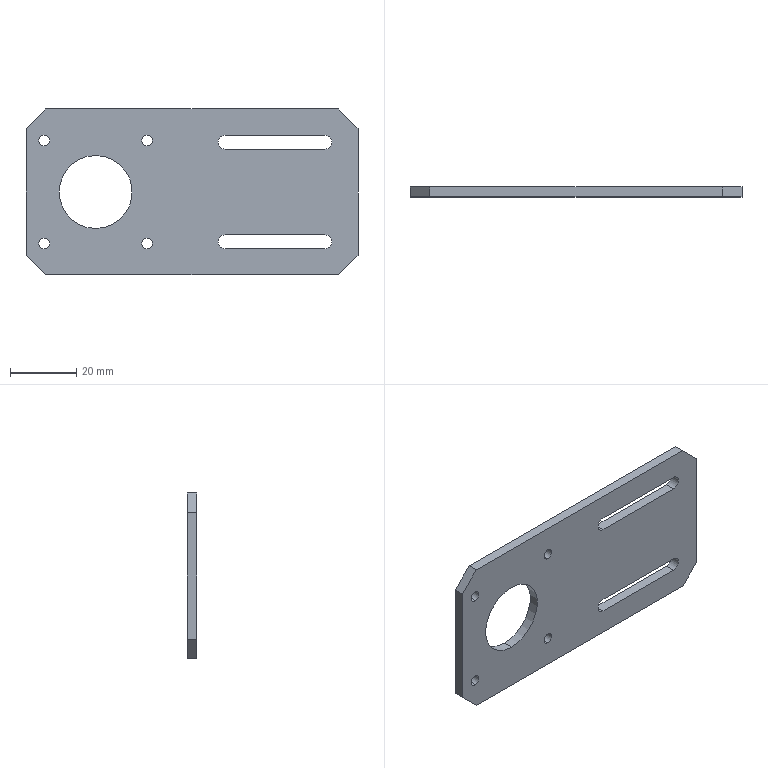Part | SolidWorks | features BaseBody 1 | 1 solid | 28 faces | box 100 x 3 x 50 mm | volume 12708 mm3 | cylinder 14 | plane 14 | commonest cylinder face diameters 3.2 x8 4.2 x4 22 x2
STEP:
#1=CARTESIAN_POINT('',(5.5,3.,-11.1));
#2=VERTEX_POINT('',#1);
#3=CARTESIAN_POINT('',(5.5,3.,-7.9));
#4=VERTEX_POINT('',#3);
#5=CARTESIAN_POINT('',(5.5,3.,-9.5));
#6=DIRECTION('',(0.,1.,0.));
#7=DIRECTION('',(0.,0.,-1.));
#8=AXIS2_PLACEMENT_3D('',#5,#6,#7);
#9=CIRCLE('',#8,1.6);
#10=EDGE_CURVE('',#2,#4,#9,.T.);
#11=ORIENTED_EDGE('',*,*,#10,.T.);
#12=CARTESIAN_POINT('',(5.5,0.,-7.9));
#13=VERTEX_POINT('',#12);
#14=CARTESIAN_POINT('',(5.5,3.,-7.9));
#15=DIRECTION('',(0.,-1.,0.));
#16=VECTOR('',#15,1000.);
#17=LINE('',#14,#16);
#18=EDGE_CURVE('',#4,#13,#17,.T.);
#19=ORIENTED_EDGE('',*,*,#18,.T.);
#20=CARTESIAN_POINT('',(5.5,0.,-11.1));
#21=VERTEX_POINT('',#20);
#22=CARTESIAN_POINT('',(5.5,0.,-9.5));
#23=DIRECTION('',(0.,1.,0.));
#24=DIRECTION('',(0.,0.,-1.));
#25=AXIS2_PLACEMENT_3D('',#22,#23,#24);
#26=CIRCLE('',#25,1.6);
#27=EDGE_CURVE('',#21,#13,#26,.T.);
#28=ORIENTED_EDGE('',*,*,#27,.F.);
#29=CARTESIAN_POINT('',(5.5,3.,-11.1));
#30=DIRECTION('',(0.,-1.,0.));
#31=VECTOR('',#30,1000.);
#32=LINE('',#29,#31);
#33=EDGE_CURVE('',#2,#21,#32,.T.);
#34=ORIENTED_EDGE('',*,*,#33,.F.);
#35=EDGE_LOOP('',(#11,#19,#28,#34));
#36=FACE_OUTER_BOUND('',#35,.T.);
#37=CARTESIAN_POINT('',(5.5,3.,-9.5));
#38=DIRECTION('',(0.,-1.,0.));
#39=DIRECTION('',(0.,0.,-1.));
#40=AXIS2_PLACEMENT_3D('',#37,#38,#39);
#41=CYLINDRICAL_SURFACE('',#40,1.6);
#42=ADVANCED_FACE('',(#36),#41,.F.);
#43=CARTESIAN_POINT('',(36.5,3.,-11.1));
#44=VERTEX_POINT('',#43);
#45=CARTESIAN_POINT('',(36.5,3.,-7.9));
#46=VERTEX_POINT('',#45);
#47=CARTESIAN_POINT('',(36.5,3.,-9.5));
#48=DIRECTION('',(0.,1.,0.));
#49=DIRECTION('',(0.,0.,-1.));
#50=AXIS2_PLACEMENT_3D('',#47,#48,#49);
#51=CIRCLE('',#50,1.6);
#52=EDGE_CURVE('',#44,#46,#51,.T.);
#53=ORIENTED_EDGE('',*,*,#52,.T.);
#54=CARTESIAN_POINT('',(36.5,0.,-7.9));
#55=VERTEX_POINT('',#54);
#56=CARTESIAN_POINT('',(36.5,3.,-7.9));
#57=DIRECTION('',(0.,-1.,0.));
#58=VECTOR('',#57,1000.);
#59=LINE('',#56,#58);
#60=EDGE_CURVE('',#46,#55,#59,.T.);
#61=ORIENTED_EDGE('',*,*,#60,.T.);
#62=CARTESIAN_POINT('',(36.5,0.,-11.1));
#63=VERTEX_POINT('',#62);
#64=CARTESIAN_POINT('',(36.5,0.,-9.5));
#65=DIRECTION('',(0.,1.,0.));
#66=DIRECTION('',(0.,0.,-1.));
#67=AXIS2_PLACEMENT_3D('',#64,#65,#66);
#68=CIRCLE('',#67,1.6);
#69=EDGE_CURVE('',#63,#55,#68,.T.);
#70=ORIENTED_EDGE('',*,*,#69,.F.);
#71=CARTESIAN_POINT('',(36.5,3.,-11.1));
#72=DIRECTION('',(0.,-1.,0.));
#73=VECTOR('',#72,1000.);
#74=LINE('',#71,#73);
#75=EDGE_CURVE('',#44,#63,#74,.T.);
#76=ORIENTED_EDGE('',*,*,#75,.F.);
#77=EDGE_LOOP('',(#53,#61,#70,#76));
#78=FACE_OUTER_BOUND('',#77,.T.);
#79=CARTESIAN_POINT('',(36.5,3.,-9.5));
#80=DIRECTION('',(0.,-1.,0.));
#81=DIRECTION('',(0.,0.,-1.));
#82=AXIS2_PLACEMENT_3D('',#79,#80,#81);
#83=CYLINDRICAL_SURFACE('',#82,1.6);
#84=ADVANCED_FACE('',(#78),#83,.F.);
#85=CARTESIAN_POINT('',(36.5,3.,-42.1));
#86=VERTEX_POINT('',#85);
#87=CARTESIAN_POINT('',(36.5,3.,-38.9));
#88=VERTEX_POINT('',#87);
#89=CARTESIAN_POINT('',(36.5,3.,-40.5));
#90=DIRECTION('',(0.,1.,0.));
#91=DIRECTION('',(0.,0.,-1.));
#92=AXIS2_PLACEMENT_3D('',#89,#90,#91);
#93=CIRCLE('',#92,1.6);
#94=EDGE_CURVE('',#86,#88,#93,.T.);
#95=ORIENTED_EDGE('',*,*,#94,.T.);
#96=CARTESIAN_POINT('',(36.5,0.,-38.9));
#97=VERTEX_POINT('',#96);
#98=CARTESIAN_POINT('',(36.5,3.,-38.9));
#99=DIRECTION('',(0.,-1.,0.));
#100=VECTOR('',#99,1000.);
#101=LINE('',#98,#100);
#102=EDGE_CURVE('',#88,#97,#101,.T.);
#103=ORIENTED_EDGE('',*,*,#102,.T.);
#104=CARTESIAN_POINT('',(36.5,0.,-42.1));
#105=VERTEX_POINT('',#104);
#106=CARTESIAN_POINT('',(36.5,0.,-40.5));
#107=DIRECTION('',(0.,1.,0.));
#108=DIRECTION('',(0.,0.,-1.));
#109=AXIS2_PLACEMENT_3D('',#106,#107,#108);
#110=CIRCLE('',#109,1.6);
#111=EDGE_CURVE('',#105,#97,#110,.T.);
#112=ORIENTED_EDGE('',*,*,#111,.F.);
#113=CARTESIAN_POINT('',(36.5,3.,-42.1));
#114=DIRECTION('',(0.,-1.,0.));
#115=VECTOR('',#114,1000.);
#116=LINE('',#113,#115);
#117=EDGE_CURVE('',#86,#105,#116,.T.);
#118=ORIENTED_EDGE('',*,*,#117,.F.);
#119=EDGE_LOOP('',(#95,#103,#112,#118));
#120=FACE_OUTER_BOUND('',#119,.T.);
#121=CARTESIAN_POINT('',(36.5,3.,-40.5));
#122=DIRECTION('',(0.,-1.,0.));
#123=DIRECTION('',(0.,0.,-1.));
#124=AXIS2_PLACEMENT_3D('',#121,#122,#123);
#125=CYLINDRICAL_SURFACE('',#124,1.6);
#126=ADVANCED_FACE('',(#120),#125,.F.);
#127=CARTESIAN_POINT('',(5.5,3.,-42.1));
#128=VERTEX_POINT('',#127);
#129=CARTESIAN_POINT('',(5.5,3.,-38.9));
#130=VERTEX_POINT('',#129);
#131=CARTESIAN_POINT('',(5.5,3.,-40.5));
#132=DIRECTION('',(0.,1.,0.));
#133=DIRECTION('',(0.,0.,-1.));
#134=AXIS2_PLACEMENT_3D('',#131,#132,#133);
#135=CIRCLE('',#134,1.6);
#136=EDGE_CURVE('',#128,#130,#135,.T.);
#137=ORIENTED_EDGE('',*,*,#136,.T.);
#138=CARTESIAN_POINT('',(5.5,0.,-38.9));
#139=VERTEX_POINT('',#138);
#140=CARTESIAN_POINT('',(5.5,3.,-38.9));
#141=DIRECTION('',(0.,-1.,0.));
#142=VECTOR('',#141,1000.);
#143=LINE('',#140,#142);
#144=EDGE_CURVE('',#130,#139,#143,.T.);
#145=ORIENTED_EDGE('',*,*,#144,.T.);
#146=CARTESIAN_POINT('',(5.5,0.,-42.1));
#147=VERTEX_POINT('',#146);
#148=CARTESIAN_POINT('',(5.5,0.,-40.5));
#149=DIRECTION('',(0.,1.,0.));
#150=DIRECTION('',(0.,0.,-1.));
#151=AXIS2_PLACEMENT_3D('',#148,#149,#150);
#152=CIRCLE('',#151,1.6);
#153=EDGE_CURVE('',#147,#139,#152,.T.);
#154=ORIENTED_EDGE('',*,*,#153,.F.);
#155=CARTESIAN_POINT('',(5.5,3.,-42.1));
#156=DIRECTION('',(0.,-1.,0.));
#157=VECTOR('',#156,1000.);
#158=LINE('',#155,#157);
#159=EDGE_CURVE('',#128,#147,#158,.T.);
#160=ORIENTED_EDGE('',*,*,#159,.F.);
#161=EDGE_LOOP('',(#137,#145,#154,#160));
#162=FACE_OUTER_BOUND('',#161,.T.);
#163=CARTESIAN_POINT('',(5.5,3.,-40.5));
#164=DIRECTION('',(0.,-1.,0.));
#165=DIRECTION('',(0.,0.,-1.));
#166=AXIS2_PLACEMENT_3D('',#163,#164,#165);
#167=CYLINDRICAL_SURFACE('',#166,1.6);
#168=ADVANCED_FACE('',(#162),#167,.F.);
#169=CARTESIAN_POINT('',(21.,3.,-36.));
#170=VERTEX_POINT('',#169);
#171=CARTESIAN_POINT('',(21.,3.,-14.));
#172=VERTEX_POINT('',#171);
#173=CARTESIAN_POINT('',(21.,3.,-25.));
#174=DIRECTION('',(0.,1.,0.));
#175=DIRECTION('',(0.,0.,-1.));
#176=AXIS2_PLACEMENT_3D('',#173,#174,#175);
#177=CIRCLE('',#176,11.);
#178=EDGE_CURVE('',#170,#172,#177,.T.);
#179=ORIENTED_EDGE('',*,*,#178,.T.);
#180=CARTESIAN_POINT('',(21.,0.,-14.));
#181=VERTEX_POINT('',#180);
#182=CARTESIAN_POINT('',(21.,3.,-14.));
#183=DIRECTION('',(0.,-1.,0.));
#184=VECTOR('',#183,1000.);
#185=LINE('',#182,#184);
#186=EDGE_CURVE('',#172,#181,#185,.T.);
#187=ORIENTED_EDGE('',*,*,#186,.T.);
#188=CARTESIAN_POINT('',(21.,0.,-36.));
#189=VERTEX_POINT('',#188);
#190=CARTESIAN_POINT('',(21.,0.,-25.));
#191=DIRECTION('',(0.,1.,0.));
#192=DIRECTION('',(0.,0.,-1.));
#193=AXIS2_PLACEMENT_3D('',#190,#191,#192);
#194=CIRCLE('',#193,11.);
#195=EDGE_CURVE('',#189,#181,#194,.T.);
#196=ORIENTED_EDGE('',*,*,#195,.F.);
#197=CARTESIAN_POINT('',(21.,3.,-36.));
#198=DIRECTION('',(0.,-1.,0.));
#199=VECTOR('',#198,1000.);
#200=LINE('',#197,#199);
#201=EDGE_CURVE('',#170,#189,#200,.T.);
#202=ORIENTED_EDGE('',*,*,#201,.F.);
#203=EDGE_LOOP('',(#179,#187,#196,#202));
#204=FACE_OUTER_BOUND('',#203,.T.);
#205=CARTESIAN_POINT('',(21.,3.,-25.));
#206=DIRECTION('',(0.,-1.,0.));
#207=DIRECTION('',(0.,0.,-1.));
#208=AXIS2_PLACEMENT_3D('',#205,#206,#207);
#209=CYLINDRICAL_SURFACE('',#208,11.);
#210=ADVANCED_FACE('',(#204),#209,.F.);
#211=CARTESIAN_POINT('',(90.,3.,-12.1));
#212=VERTEX_POINT('',#211);
#213=CARTESIAN_POINT('',(60.,3.,-12.1));
#214=VERTEX_POINT('',#213);
#215=CARTESIAN_POINT('',(0.,3.,-12.1));
#216=DIRECTION('',(-1.,0.,0.));
#217=VECTOR('',#216,1000.);
#218=LINE('',#215,#217);
#219=EDGE_CURVE('',#212,#214,#218,.T.);
#220=ORIENTED_EDGE('',*,*,#219,.F.);
#221=CARTESIAN_POINT('',(90.,3.,-7.9));
#222=VERTEX_POINT('',#221);
#223=CARTESIAN_POINT('',(90.,3.,-10.));
#224=DIRECTION('',(0.,1.,0.));
#225=DIRECTION('',(0.,0.,-1.));
#226=AXIS2_PLACEMENT_3D('',#223,#224,#225);
#227=CIRCLE('',#226,2.1);
#228=EDGE_CURVE('',#222,#212,#227,.T.);
#229=ORIENTED_EDGE('',*,*,#228,.F.);
#230=CARTESIAN_POINT('',(60.,3.,-7.9));
#231=VERTEX_POINT('',#230);
#232=CARTESIAN_POINT('',(0.,3.,-7.9));
#233=DIRECTION('',(1.,0.,0.));
#234=VECTOR('',#233,1000.);
#235=LINE('',#232,#234);
#236=EDGE_CURVE('',#231,#222,#235,.T.);
#237=ORIENTED_EDGE('',*,*,#236,.F.);
#238=CARTESIAN_POINT('',(60.,3.,-10.));
#239=DIRECTION('',(0.,1.,0.));
#240=DIRECTION('',(0.,0.,-1.));
#241=AXIS2_PLACEMENT_3D('',#238,#239,#240);
#242=CIRCLE('',#241,2.1);
#243=EDGE_CURVE('',#214,#231,#242,.T.);
#244=ORIENTED_EDGE('',*,*,#243,.F.);
#245=EDGE_LOOP('',(#220,#229,#237,#244));
#246=FACE_BOUND('',#245,.T.);
#247=ORIENTED_EDGE('',*,*,#10,.F.);
#248=CARTESIAN_POINT('',(5.5,3.,-9.5));
#249=DIRECTION('',(0.,1.,0.));
#250=DIRECTION('',(0.,0.,-1.));
#251=AXIS2_PLACEMENT_3D('',#248,#249,#250);
#252=CIRCLE('',#251,1.6);
#253=EDGE_CURVE('',#4,#2,#252,.T.);
#254=ORIENTED_EDGE('',*,*,#253,.F.);
#255=EDGE_LOOP('',(#247,#254));
#256=FACE_BOUND('',#255,.T.);
#257=ORIENTED_EDGE('',*,*,#52,.F.);
#258=CARTESIAN_POINT('',(36.5,3.,-9.5));
#259=DIRECTION('',(0.,1.,0.));
#260=DIRECTION('',(0.,0.,-1.));
#261=AXIS2_PLACEMENT_3D('',#258,#259,#260);
#262=CIRCLE('',#261,1.6);
#263=EDGE_CURVE('',#46,#44,#262,.T.);
#264=ORIENTED_EDGE('',*,*,#263,.F.);
#265=EDGE_LOOP('',(#257,#264));
#266=FACE_BOUND('',#265,.T.);
#267=ORIENTED_EDGE('',*,*,#94,.F.);
#268=CARTESIAN_POINT('',(36.5,3.,-40.5));
#269=DIRECTION('',(0.,1.,0.));
#270=DIRECTION('',(0.,0.,-1.));
#271=AXIS2_PLACEMENT_3D('',#268,#269,#270);
#272=CIRCLE('',#271,1.6);
#273=EDGE_CURVE('',#88,#86,#272,.T.);
#274=ORIENTED_EDGE('',*,*,#273,.F.);
#275=EDGE_LOOP('',(#267,#274));
#276=FACE_BOUND('',#275,.T.);
#277=ORIENTED_EDGE('',*,*,#136,.F.);
#278=CARTESIAN_POINT('',(5.5,3.,-40.5));
#279=DIRECTION('',(0.,1.,0.));
#280=DIRECTION('',(0.,0.,-1.));
#281=AXIS2_PLACEMENT_3D('',#278,#279,#280);
#282=CIRCLE('',#281,1.6);
#283=EDGE_CURVE('',#130,#128,#282,.T.);
#284=ORIENTED_EDGE('',*,*,#283,.F.);
#285=EDGE_LOOP('',(#277,#284));
#286=FACE_BOUND('',#285,.T.);
#287=ORIENTED_EDGE('',*,*,#178,.F.);
#288=CARTESIAN_POINT('',(21.,3.,-25.));
#289=DIRECTION('',(0.,1.,0.));
#290=DIRECTION('',(0.,0.,-1.));
#291=AXIS2_PLACEMENT_3D('',#288,#289,#290);
#292=CIRCLE('',#291,11.);
#293=EDGE_CURVE('',#172,#170,#292,.T.);
#294=ORIENTED_EDGE('',*,*,#293,.F.);
#295=EDGE_LOOP('',(#287,#294));
#296=FACE_BOUND('',#295,.T.);
#297=CARTESIAN_POINT('',(6.,3.,0.));
#298=VERTEX_POINT('',#297);
#299=CARTESIAN_POINT('',(0.,3.,-6.));
#300=VERTEX_POINT('',#299);
#301=CARTESIAN_POINT('',(6.,3.,0.));
#302=DIRECTION('',(-0.7071,0.,-0.7071));
#303=VECTOR('',#302,1000.);
#304=LINE('',#301,#303);
#305=EDGE_CURVE('',#298,#300,#304,.T.);
#306=ORIENTED_EDGE('',*,*,#305,.F.);
#307=CARTESIAN_POINT('',(94.,3.,0.));
#308=VERTEX_POINT('',#307);
#309=CARTESIAN_POINT('',(0.,3.,0.));
#310=DIRECTION('',(-1.,0.,0.));
#311=VECTOR('',#310,1000.);
#312=LINE('',#309,#311);
#313=EDGE_CURVE('',#308,#298,#312,.T.);
#314=ORIENTED_EDGE('',*,*,#313,.F.);
#315=CARTESIAN_POINT('',(100.,3.,-6.));
#316=VERTEX_POINT('',#315);
#317=CARTESIAN_POINT('',(100.,3.,-6.));
#318=DIRECTION('',(-0.7071,0.,0.7071));
#319=VECTOR('',#318,1000.);
#320=LINE('',#317,#319);
#321=EDGE_CURVE('',#316,#308,#320,.T.);
#322=ORIENTED_EDGE('',*,*,#321,.F.);
#323=CARTESIAN_POINT('',(100.,3.,-44.));
#324=VERTEX_POINT('',#323);
#325=CARTESIAN_POINT('',(100.,3.,0.));
#326=DIRECTION('',(0.,0.,1.));
#327=VECTOR('',#326,1000.);
#328=LINE('',#325,#327);
#329=EDGE_CURVE('',#324,#316,#328,.T.);
#330=ORIENTED_EDGE('',*,*,#329,.F.);
#331=CARTESIAN_POINT('',(94.,3.,-50.));
#332=VERTEX_POINT('',#331);
#333=CARTESIAN_POINT('',(94.,3.,-50.));
#334=DIRECTION('',(0.7071,0.,0.7071));
#335=VECTOR('',#334,1000.);
#336=LINE('',#333,#335);
#337=EDGE_CURVE('',#332,#324,#336,.T.);
#338=ORIENTED_EDGE('',*,*,#337,.F.);
#339=CARTESIAN_POINT('',(6.,3.,-50.));
#340=VERTEX_POINT('',#339);
#341=CARTESIAN_POINT('',(0.,3.,-50.));
#342=DIRECTION('',(1.,0.,0.));
#343=VECTOR('',#342,1000.);
#344=LINE('',#341,#343);
#345=EDGE_CURVE('',#340,#332,#344,.T.);
#346=ORIENTED_EDGE('',*,*,#345,.F.);
#347=CARTESIAN_POINT('',(0.,3.,-44.));
#348=VERTEX_POINT('',#347);
#349=CARTESIAN_POINT('',(0.,3.,-44.));
#350=DIRECTION('',(0.7071,0.,-0.7071));
#351=VECTOR('',#350,1000.);
#352=LINE('',#349,#351);
#353=EDGE_CURVE('',#348,#340,#352,.T.);
#354=ORIENTED_EDGE('',*,*,#353,.F.);
#355=CARTESIAN_POINT('',(0.,3.,0.));
#356=DIRECTION('',(0.,0.,-1.));
#357=VECTOR('',#356,1000.);
#358=LINE('',#355,#357);
#359=EDGE_CURVE('',#300,#348,#358,.T.);
#360=ORIENTED_EDGE('',*,*,#359,.F.);
#361=EDGE_LOOP('',(#306,#314,#322,#330,#338,#346,#354,#360));
#362=FACE_OUTER_BOUND('',#361,.T.);
#363=CARTESIAN_POINT('',(90.,3.,-42.1));
#364=VERTEX_POINT('',#363);
#365=CARTESIAN_POINT('',(60.,3.,-42.1));
#366=VERTEX_POINT('',#365);
#367=CARTESIAN_POINT('',(0.,3.,-42.1));
#368=DIRECTION('',(-1.,0.,0.));
#369=VECTOR('',#368,1000.);
#370=LINE('',#367,#369);
#371=EDGE_CURVE('',#364,#366,#370,.T.);
#372=ORIENTED_EDGE('',*,*,#371,.F.);
#373=CARTESIAN_POINT('',(90.,3.,-37.9));
#374=VERTEX_POINT('',#373);
#375=CARTESIAN_POINT('',(90.,3.,-40.));
#376=DIRECTION('',(0.,1.,0.));
#377=DIRECTION('',(0.,0.,-1.));
#378=AXIS2_PLACEMENT_3D('',#375,#376,#377);
#379=CIRCLE('',#378,2.1);
#380=EDGE_CURVE('',#374,#364,#379,.T.);
#381=ORIENTED_EDGE('',*,*,#380,.F.);
#382=CARTESIAN_POINT('',(60.,3.,-37.9));
#383=VERTEX_POINT('',#382);
#384=CARTESIAN_POINT('',(0.,3.,-37.9));
#385=DIRECTION('',(1.,0.,0.));
#386=VECTOR('',#385,1000.);
#387=LINE('',#384,#386);
#388=EDGE_CURVE('',#383,#374,#387,.T.);
#389=ORIENTED_EDGE('',*,*,#388,.F.);
#390=CARTESIAN_POINT('',(60.,3.,-40.));
#391=DIRECTION('',(0.,1.,0.));
#392=DIRECTION('',(0.,0.,-1.));
#393=AXIS2_PLACEMENT_3D('',#390,#391,#392);
#394=CIRCLE('',#393,2.1);
#395=EDGE_CURVE('',#366,#383,#394,.T.);
#396=ORIENTED_EDGE('',*,*,#395,.F.);
#397=EDGE_LOOP('',(#372,#381,#389,#396));
#398=FACE_BOUND('',#397,.T.);
#399=CARTESIAN_POINT('',(0.,3.,0.));
#400=DIRECTION('',(0.,-1.,0.));
#401=DIRECTION('',(0.,0.,-1.));
#402=AXIS2_PLACEMENT_3D('',#399,#400,#401);
#403=PLANE('',#402);
#404=ADVANCED_FACE('',(#246,#256,#266,#276,#286,#296,#362,#398),#403,.F.);
#405=CARTESIAN_POINT('',(60.,0.,-12.1));
#406=VERTEX_POINT('',#405);
#407=CARTESIAN_POINT('',(60.,3.,-12.1));
#408=DIRECTION('',(0.,-1.,0.));
#409=VECTOR('',#408,1000.);
#410=LINE('',#407,#409);
#411=EDGE_CURVE('',#214,#406,#410,.T.);
#412=ORIENTED_EDGE('',*,*,#411,.F.);
#413=ORIENTED_EDGE('',*,*,#243,.T.);
#414=CARTESIAN_POINT('',(60.,0.,-7.9));
#415=VERTEX_POINT('',#414);
#416=CARTESIAN_POINT('',(60.,3.,-7.9));
#417=DIRECTION('',(0.,1.,0.));
#418=VECTOR('',#417,1000.);
#419=LINE('',#416,#418);
#420=EDGE_CURVE('',#415,#231,#419,.T.);
#421=ORIENTED_EDGE('',*,*,#420,.F.);
#422=CARTESIAN_POINT('',(60.,0.,-10.));
#423=DIRECTION('',(0.,1.,0.));
#424=DIRECTION('',(0.,0.,-1.));
#425=AXIS2_PLACEMENT_3D('',#422,#423,#424);
#426=CIRCLE('',#425,2.1);
#427=EDGE_CURVE('',#406,#415,#426,.T.);
#428=ORIENTED_EDGE('',*,*,#427,.F.);
#429=EDGE_LOOP('',(#412,#413,#421,#428));
#430=FACE_OUTER_BOUND('',#429,.T.);
#431=CARTESIAN_POINT('',(60.,3.,-10.));
#432=DIRECTION('',(0.,-1.,0.));
#433=DIRECTION('',(0.,0.,-1.));
#434=AXIS2_PLACEMENT_3D('',#431,#432,#433);
#435=CYLINDRICAL_SURFACE('',#434,2.1);
#436=ADVANCED_FACE('',(#430),#435,.F.);
#437=ORIENTED_EDGE('',*,*,#219,.T.);
#438=ORIENTED_EDGE('',*,*,#411,.T.);
#439=CARTESIAN_POINT('',(90.,0.,-12.1));
#440=VERTEX_POINT('',#439);
#441=CARTESIAN_POINT('',(60.,0.,-12.1));
#442=DIRECTION('',(1.,0.,0.));
#443=VECTOR('',#442,1000.);
#444=LINE('',#441,#443);
#445=EDGE_CURVE('',#406,#440,#444,.T.);
#446=ORIENTED_EDGE('',*,*,#445,.T.);
#447=CARTESIAN_POINT('',(90.,3.,-12.1));
#448=DIRECTION('',(0.,1.,0.));
#449=VECTOR('',#448,1000.);
#450=LINE('',#447,#449);
#451=EDGE_CURVE('',#440,#212,#450,.T.);
#452=ORIENTED_EDGE('',*,*,#451,.T.);
#453=EDGE_LOOP('',(#437,#438,#446,#452));
#454=FACE_OUTER_BOUND('',#453,.T.);
#455=CARTESIAN_POINT('',(60.,3.,-12.1));
#456=DIRECTION('',(0.,0.,1.));
#457=DIRECTION('',(1.,0.,0.));
#458=AXIS2_PLACEMENT_3D('',#455,#456,#457);
#459=PLANE('',#458);
#460=ADVANCED_FACE('',(#454),#459,.T.);
#461=CARTESIAN_POINT('',(90.,0.,-7.9));
#462=VERTEX_POINT('',#461);
#463=CARTESIAN_POINT('',(90.,3.,-7.9));
#464=DIRECTION('',(0.,-1.,0.));
#465=VECTOR('',#464,1000.);
#466=LINE('',#463,#465);
#467=EDGE_CURVE('',#222,#462,#466,.T.);
#468=ORIENTED_EDGE('',*,*,#467,.F.);
#469=ORIENTED_EDGE('',*,*,#228,.T.);
#470=ORIENTED_EDGE('',*,*,#451,.F.);
#471=CARTESIAN_POINT('',(90.,0.,-10.));
#472=DIRECTION('',(0.,1.,0.));
#473=DIRECTION('',(0.,0.,-1.));
#474=AXIS2_PLACEMENT_3D('',#471,#472,#473);
#475=CIRCLE('',#474,2.1);
#476=EDGE_CURVE('',#462,#440,#475,.T.);
#477=ORIENTED_EDGE('',*,*,#476,.F.);
#478=EDGE_LOOP('',(#468,#469,#470,#477));
#479=FACE_OUTER_BOUND('',#478,.T.);
#480=CARTESIAN_POINT('',(90.,3.,-10.));
#481=DIRECTION('',(0.,-1.,0.));
#482=DIRECTION('',(0.,0.,-1.));
#483=AXIS2_PLACEMENT_3D('',#480,#481,#482);
#484=CYLINDRICAL_SURFACE('',#483,2.1);
#485=ADVANCED_FACE('',(#479),#484,.F.);
#486=ORIENTED_EDGE('',*,*,#236,.T.);
#487=ORIENTED_EDGE('',*,*,#467,.T.);
#488=CARTESIAN_POINT('',(60.,0.,-7.9));
#489=DIRECTION('',(-1.,0.,0.));
#490=VECTOR('',#489,1000.);
#491=LINE('',#488,#490);
#492=EDGE_CURVE('',#462,#415,#491,.T.);
#493=ORIENTED_EDGE('',*,*,#492,.T.);
#494=ORIENTED_EDGE('',*,*,#420,.T.);
#495=EDGE_LOOP('',(#486,#487,#493,#494));
#496=FACE_OUTER_BOUND('',#495,.T.);
#497=CARTESIAN_POINT('',(60.,3.,-7.9));
#498=DIRECTION('',(0.,0.,-1.));
#499=DIRECTION('',(-1.,0.,0.));
#500=AXIS2_PLACEMENT_3D('',#497,#498,#499);
#501=PLANE('',#500);
#502=ADVANCED_FACE('',(#496),#501,.T.);
#503=ORIENTED_EDGE('',*,*,#18,.F.);
#504=ORIENTED_EDGE('',*,*,#253,.T.);
#505=ORIENTED_EDGE('',*,*,#33,.T.);
#506=CARTESIAN_POINT('',(5.5,0.,-9.5));
#507=DIRECTION('',(0.,1.,0.));
#508=DIRECTION('',(0.,0.,-1.));
#509=AXIS2_PLACEMENT_3D('',#506,#507,#508);
#510=CIRCLE('',#509,1.6);
#511=EDGE_CURVE('',#13,#21,#510,.T.);
#512=ORIENTED_EDGE('',*,*,#511,.F.);
#513=EDGE_LOOP('',(#503,#504,#505,#512));
#514=FACE_OUTER_BOUND('',#513,.T.);
#515=CARTESIAN_POINT('',(5.5,3.,-9.5));
#516=DIRECTION('',(0.,-1.,0.));
#517=DIRECTION('',(0.,0.,-1.));
#518=AXIS2_PLACEMENT_3D('',#515,#516,#517);
#519=CYLINDRICAL_SURFACE('',#518,1.6);
#520=ADVANCED_FACE('',(#514),#519,.F.);
#521=ORIENTED_EDGE('',*,*,#60,.F.);
#522=ORIENTED_EDGE('',*,*,#263,.T.);
#523=ORIENTED_EDGE('',*,*,#75,.T.);
#524=CARTESIAN_POINT('',(36.5,0.,-9.5));
#525=DIRECTION('',(0.,1.,0.));
#526=DIRECTION('',(0.,0.,-1.));
#527=AXIS2_PLACEMENT_3D('',#524,#525,#526);
#528=CIRCLE('',#527,1.6);
#529=EDGE_CURVE('',#55,#63,#528,.T.);
#530=ORIENTED_EDGE('',*,*,#529,.F.);
#531=EDGE_LOOP('',(#521,#522,#523,#530));
#532=FACE_OUTER_BOUND('',#531,.T.);
#533=CARTESIAN_POINT('',(36.5,3.,-9.5));
#534=DIRECTION('',(0.,-1.,0.));
#535=DIRECTION('',(0.,0.,-1.));
#536=AXIS2_PLACEMENT_3D('',#533,#534,#535);
#537=CYLINDRICAL_SURFACE('',#536,1.6);
#538=ADVANCED_FACE('',(#532),#537,.F.);
#539=ORIENTED_EDGE('',*,*,#102,.F.);
#540=ORIENTED_EDGE('',*,*,#273,.T.);
#541=ORIENTED_EDGE('',*,*,#117,.T.);
#542=CARTESIAN_POINT('',(36.5,0.,-40.5));
#543=DIRECTION('',(0.,1.,0.));
#544=DIRECTION('',(0.,0.,-1.));
#545=AXIS2_PLACEMENT_3D('',#542,#543,#544);
#546=CIRCLE('',#545,1.6);
#547=EDGE_CURVE('',#97,#105,#546,.T.);
#548=ORIENTED_EDGE('',*,*,#547,.F.);
#549=EDGE_LOOP('',(#539,#540,#541,#548));
#550=FACE_OUTER_BOUND('',#549,.T.);
#551=CARTESIAN_POINT('',(36.5,3.,-40.5));
#552=DIRECTION('',(0.,-1.,0.));
#553=DIRECTION('',(0.,0.,-1.));
#554=AXIS2_PLACEMENT_3D('',#551,#552,#553);
#555=CYLINDRICAL_SURFACE('',#554,1.6);
#556=ADVANCED_FACE('',(#550),#555,.F.);
#557=ORIENTED_EDGE('',*,*,#144,.F.);
#558=ORIENTED_EDGE('',*,*,#283,.T.);
#559=ORIENTED_EDGE('',*,*,#159,.T.);
#560=CARTESIAN_POINT('',(5.5,0.,-40.5));
#561=DIRECTION('',(0.,1.,0.));
#562=DIRECTION('',(0.,0.,-1.));
#563=AXIS2_PLACEMENT_3D('',#560,#561,#562);
#564=CIRCLE('',#563,1.6);
#565=EDGE_CURVE('',#139,#147,#564,.T.);
#566=ORIENTED_EDGE('',*,*,#565,.F.);
#567=EDGE_LOOP('',(#557,#558,#559,#566));
#568=FACE_OUTER_BOUND('',#567,.T.);
#569=CARTESIAN_POINT('',(5.5,3.,-40.5));
#570=DIRECTION('',(0.,-1.,0.));
#571=DIRECTION('',(0.,0.,-1.));
#572=AXIS2_PLACEMENT_3D('',#569,#570,#571);
#573=CYLINDRICAL_SURFACE('',#572,1.6);
#574=ADVANCED_FACE('',(#568),#573,.F.);
#575=ORIENTED_EDGE('',*,*,#186,.F.);
#576=ORIENTED_EDGE('',*,*,#293,.T.);
#577=ORIENTED_EDGE('',*,*,#201,.T.);
#578=CARTESIAN_POINT('',(21.,0.,-25.));
#579=DIRECTION('',(0.,1.,0.));
#580=DIRECTION('',(0.,0.,-1.));
#581=AXIS2_PLACEMENT_3D('',#578,#579,#580);
#582=CIRCLE('',#581,11.);
#583=EDGE_CURVE('',#181,#189,#582,.T.);
#584=ORIENTED_EDGE('',*,*,#583,.F.);
#585=EDGE_LOOP('',(#575,#576,#577,#584));
#586=FACE_OUTER_BOUND('',#585,.T.);
#587=CARTESIAN_POINT('',(21.,3.,-25.));
#588=DIRECTION('',(0.,-1.,0.));
#589=DIRECTION('',(0.,0.,-1.));
#590=AXIS2_PLACEMENT_3D('',#587,#588,#589);
#591=CYLINDRICAL_SURFACE('',#590,11.);
#592=ADVANCED_FACE('',(#586),#591,.F.);
#593=CARTESIAN_POINT('',(0.,0.,-6.));
#594=VERTEX_POINT('',#593);
#595=CARTESIAN_POINT('',(0.,3.,-6.));
#596=DIRECTION('',(0.,-1.,0.));
#597=VECTOR('',#596,1000.);
#598=LINE('',#595,#597);
#599=EDGE_CURVE('',#300,#594,#598,.T.);
#600=ORIENTED_EDGE('',*,*,#599,.F.);
#601=ORIENTED_EDGE('',*,*,#359,.T.);
#602=CARTESIAN_POINT('',(0.,0.,-44.));
#603=VERTEX_POINT('',#602);
#604=CARTESIAN_POINT('',(0.,3.,-44.));
#605=DIRECTION('',(0.,1.,0.));
#606=VECTOR('',#605,1000.);
#607=LINE('',#604,#606);
#608=EDGE_CURVE('',#603,#348,#607,.T.);
#609=ORIENTED_EDGE('',*,*,#608,.F.);
#610=CARTESIAN_POINT('',(0.,0.,0.));
#611=DIRECTION('',(0.,0.,-1.));
#612=VECTOR('',#611,1000.);
#613=LINE('',#610,#612);
#614=EDGE_CURVE('',#594,#603,#613,.T.);
#615=ORIENTED_EDGE('',*,*,#614,.F.);
#616=EDGE_LOOP('',(#600,#601,#609,#615));
#617=FACE_OUTER_BOUND('',#616,.T.);
#618=CARTESIAN_POINT('',(0.,3.,0.));
#619=DIRECTION('',(1.,0.,0.));
#620=DIRECTION('',(0.,0.,-1.));
#621=AXIS2_PLACEMENT_3D('',#618,#619,#620);
#622=PLANE('',#621);
#623=ADVANCED_FACE('',(#617),#622,.F.);
#624=ORIENTED_EDGE('',*,*,#599,.T.);
#625=CARTESIAN_POINT('',(6.,0.,0.));
#626=VERTEX_POINT('',#625);
#627=CARTESIAN_POINT('',(6.,0.,0.));
#628=DIRECTION('',(-0.7071,0.,-0.7071));
#629=VECTOR('',#628,1000.);
#630=LINE('',#627,#629);
#631=EDGE_CURVE('',#626,#594,#630,.T.);
#632=ORIENTED_EDGE('',*,*,#631,.F.);
#633=CARTESIAN_POINT('',(6.,3.,0.));
#634=DIRECTION('',(0.,-1.,0.));
#635=VECTOR('',#634,1000.);
#636=LINE('',#633,#635);
#637=EDGE_CURVE('',#298,#626,#636,.T.);
#638=ORIENTED_EDGE('',*,*,#637,.F.);
#639=ORIENTED_EDGE('',*,*,#305,.T.);
#640=EDGE_LOOP('',(#624,#632,#638,#639));
#641=FACE_OUTER_BOUND('',#640,.T.);
#642=CARTESIAN_POINT('',(6.,3.,0.));
#643=DIRECTION('',(0.7071,0.,-0.7071));
#644=DIRECTION('',(-0.7071,0.,-0.7071));
#645=AXIS2_PLACEMENT_3D('',#642,#643,#644);
#646=PLANE('',#645);
#647=ADVANCED_FACE('',(#641),#646,.F.);
#648=ORIENTED_EDGE('',*,*,#637,.T.);
#649=CARTESIAN_POINT('',(94.,0.,0.));
#650=VERTEX_POINT('',#649);
#651=CARTESIAN_POINT('',(0.,0.,0.));
#652=DIRECTION('',(-1.,0.,0.));
#653=VECTOR('',#652,1000.);
#654=LINE('',#651,#653);
#655=EDGE_CURVE('',#650,#626,#654,.T.);
#656=ORIENTED_EDGE('',*,*,#655,.F.);
#657=CARTESIAN_POINT('',(94.,3.,0.));
#658=DIRECTION('',(0.,-1.,0.));
#659=VECTOR('',#658,1000.);
#660=LINE('',#657,#659);
#661=EDGE_CURVE('',#308,#650,#660,.T.);
#662=ORIENTED_EDGE('',*,*,#661,.F.);
#663=ORIENTED_EDGE('',*,*,#313,.T.);
#664=EDGE_LOOP('',(#648,#656,#662,#663));
#665=FACE_OUTER_BOUND('',#664,.T.);
#666=CARTESIAN_POINT('',(0.,3.,0.));
#667=DIRECTION('',(0.,0.,-1.));
#668=DIRECTION('',(-1.,0.,0.));
#669=AXIS2_PLACEMENT_3D('',#666,#667,#668);
#670=PLANE('',#669);
#671=ADVANCED_FACE('',(#665),#670,.F.);
#672=ORIENTED_EDGE('',*,*,#661,.T.);
#673=CARTESIAN_POINT('',(100.,0.,-6.));
#674=VERTEX_POINT('',#673);
#675=CARTESIAN_POINT('',(100.,0.,-6.));
#676=DIRECTION('',(-0.7071,0.,0.7071));
#677=VECTOR('',#676,1000.);
#678=LINE('',#675,#677);
#679=EDGE_CURVE('',#674,#650,#678,.T.);
#680=ORIENTED_EDGE('',*,*,#679,.F.);
#681=CARTESIAN_POINT('',(100.,3.,-6.));
#682=DIRECTION('',(0.,-1.,0.));
#683=VECTOR('',#682,1000.);
#684=LINE('',#681,#683);
#685=EDGE_CURVE('',#316,#674,#684,.T.);
#686=ORIENTED_EDGE('',*,*,#685,.F.);
#687=ORIENTED_EDGE('',*,*,#321,.T.);
#688=EDGE_LOOP('',(#672,#680,#686,#687));
#689=FACE_OUTER_BOUND('',#688,.T.);
#690=CARTESIAN_POINT('',(100.,3.,-6.));
#691=DIRECTION('',(-0.7071,0.,-0.7071));
#692=DIRECTION('',(-0.7071,0.,0.7071));
#693=AXIS2_PLACEMENT_3D('',#690,#691,#692);
#694=PLANE('',#693);
#695=ADVANCED_FACE('',(#689),#694,.F.);
#696=CARTESIAN_POINT('',(100.,0.,-44.));
#697=VERTEX_POINT('',#696);
#698=CARTESIAN_POINT('',(100.,3.,-44.));
#699=DIRECTION('',(0.,-1.,0.));
#700=VECTOR('',#699,1000.);
#701=LINE('',#698,#700);
#702=EDGE_CURVE('',#324,#697,#701,.T.);
#703=ORIENTED_EDGE('',*,*,#702,.F.);
#704=ORIENTED_EDGE('',*,*,#329,.T.);
#705=ORIENTED_EDGE('',*,*,#685,.T.);
#706=CARTESIAN_POINT('',(100.,0.,0.));
#707=DIRECTION('',(0.,0.,1.));
#708=VECTOR('',#707,1000.);
#709=LINE('',#706,#708);
#710=EDGE_CURVE('',#697,#674,#709,.T.);
#711=ORIENTED_EDGE('',*,*,#710,.F.);
#712=EDGE_LOOP('',(#703,#704,#705,#711));
#713=FACE_OUTER_BOUND('',#712,.T.);
#714=CARTESIAN_POINT('',(100.,3.,0.));
#715=DIRECTION('',(-1.,0.,0.));
#716=DIRECTION('',(0.,0.,1.));
#717=AXIS2_PLACEMENT_3D('',#714,#715,#716);
#718=PLANE('',#717);
#719=ADVANCED_FACE('',(#713),#718,.F.);
#720=ORIENTED_EDGE('',*,*,#702,.T.);
#721=CARTESIAN_POINT('',(94.,0.,-50.));
#722=VERTEX_POINT('',#721);
#723=CARTESIAN_POINT('',(94.,0.,-50.));
#724=DIRECTION('',(0.7071,0.,0.7071));
#725=VECTOR('',#724,1000.);
#726=LINE('',#723,#725);
#727=EDGE_CURVE('',#722,#697,#726,.T.);
#728=ORIENTED_EDGE('',*,*,#727,.F.);
#729=CARTESIAN_POINT('',(94.,3.,-50.));
#730=DIRECTION('',(0.,-1.,0.));
#731=VECTOR('',#730,1000.);
#732=LINE('',#729,#731);
#733=EDGE_CURVE('',#332,#722,#732,.T.);
#734=ORIENTED_EDGE('',*,*,#733,.F.);
#735=ORIENTED_EDGE('',*,*,#337,.T.);
#736=EDGE_LOOP('',(#720,#728,#734,#735));
#737=FACE_OUTER_BOUND('',#736,.T.);
#738=CARTESIAN_POINT('',(94.,3.,-50.));
#739=DIRECTION('',(-0.7071,0.,0.7071));
#740=DIRECTION('',(0.7071,0.,0.7071));
#741=AXIS2_PLACEMENT_3D('',#738,#739,#740);
#742=PLANE('',#741);
#743=ADVANCED_FACE('',(#737),#742,.F.);
#744=CARTESIAN_POINT('',(6.,0.,-50.));
#745=VERTEX_POINT('',#744);
#746=CARTESIAN_POINT('',(6.,3.,-50.));
#747=DIRECTION('',(0.,-1.,0.));
#748=VECTOR('',#747,1000.);
#749=LINE('',#746,#748);
#750=EDGE_CURVE('',#340,#745,#749,.T.);
#751=ORIENTED_EDGE('',*,*,#750,.F.);
#752=ORIENTED_EDGE('',*,*,#345,.T.);
#753=ORIENTED_EDGE('',*,*,#733,.T.);
#754=CARTESIAN_POINT('',(0.,0.,-50.));
#755=DIRECTION('',(1.,0.,0.));
#756=VECTOR('',#755,1000.);
#757=LINE('',#754,#756);
#758=EDGE_CURVE('',#745,#722,#757,.T.);
#759=ORIENTED_EDGE('',*,*,#758,.F.);
#760=EDGE_LOOP('',(#751,#752,#753,#759));
#761=FACE_OUTER_BOUND('',#760,.T.);
#762=CARTESIAN_POINT('',(0.,3.,-50.));
#763=DIRECTION('',(0.,0.,1.));
#764=DIRECTION('',(1.,0.,0.));
#765=AXIS2_PLACEMENT_3D('',#762,#763,#764);
#766=PLANE('',#765);
#767=ADVANCED_FACE('',(#761),#766,.F.);
#768=ORIENTED_EDGE('',*,*,#750,.T.);
#769=CARTESIAN_POINT('',(0.,0.,-44.));
#770=DIRECTION('',(0.7071,0.,-0.7071));
#771=VECTOR('',#770,1000.);
#772=LINE('',#769,#771);
#773=EDGE_CURVE('',#603,#745,#772,.T.);
#774=ORIENTED_EDGE('',*,*,#773,.F.);
#775=ORIENTED_EDGE('',*,*,#608,.T.);
#776=ORIENTED_EDGE('',*,*,#353,.T.);
#777=EDGE_LOOP('',(#768,#774,#775,#776));
#778=FACE_OUTER_BOUND('',#777,.T.);
#779=CARTESIAN_POINT('',(0.,3.,-44.));
#780=DIRECTION('',(0.7071,0.,0.7071));
#781=DIRECTION('',(0.7071,0.,-0.7071));
#782=AXIS2_PLACEMENT_3D('',#779,#780,#781);
#783=PLANE('',#782);
#784=ADVANCED_FACE('',(#778),#783,.F.);
#785=CARTESIAN_POINT('',(60.,0.,-42.1));
#786=VERTEX_POINT('',#785);
#787=CARTESIAN_POINT('',(60.,3.,-42.1));
#788=DIRECTION('',(0.,-1.,0.));
#789=VECTOR('',#788,1000.);
#790=LINE('',#787,#789);
#791=EDGE_CURVE('',#366,#786,#790,.T.);
#792=ORIENTED_EDGE('',*,*,#791,.F.);
#793=ORIENTED_EDGE('',*,*,#395,.T.);
#794=CARTESIAN_POINT('',(60.,0.,-37.9));
#795=VERTEX_POINT('',#794);
#796=CARTESIAN_POINT('',(60.,3.,-37.9));
#797=DIRECTION('',(0.,1.,0.));
#798=VECTOR('',#797,1000.);
#799=LINE('',#796,#798);
#800=EDGE_CURVE('',#795,#383,#799,.T.);
#801=ORIENTED_EDGE('',*,*,#800,.F.);
#802=CARTESIAN_POINT('',(60.,0.,-40.));
#803=DIRECTION('',(0.,1.,0.));
#804=DIRECTION('',(0.,0.,-1.));
#805=AXIS2_PLACEMENT_3D('',#802,#803,#804);
#806=CIRCLE('',#805,2.1);
#807=EDGE_CURVE('',#786,#795,#806,.T.);
#808=ORIENTED_EDGE('',*,*,#807,.F.);
#809=EDGE_LOOP('',(#792,#793,#801,#808));
#810=FACE_OUTER_BOUND('',#809,.T.);
#811=CARTESIAN_POINT('',(60.,3.,-40.));
#812=DIRECTION('',(0.,-1.,0.));
#813=DIRECTION('',(0.,0.,-1.));
#814=AXIS2_PLACEMENT_3D('',#811,#812,#813);
#815=CYLINDRICAL_SURFACE('',#814,2.1);
#816=ADVANCED_FACE('',(#810),#815,.F.);
#817=ORIENTED_EDGE('',*,*,#371,.T.);
#818=ORIENTED_EDGE('',*,*,#791,.T.);
#819=CARTESIAN_POINT('',(90.,0.,-42.1));
#820=VERTEX_POINT('',#819);
#821=CARTESIAN_POINT('',(60.,0.,-42.1));
#822=DIRECTION('',(1.,0.,0.));
#823=VECTOR('',#822,1000.);
#824=LINE('',#821,#823);
#825=EDGE_CURVE('',#786,#820,#824,.T.);
#826=ORIENTED_EDGE('',*,*,#825,.T.);
#827=CARTESIAN_POINT('',(90.,3.,-42.1));
#828=DIRECTION('',(0.,1.,0.));
#829=VECTOR('',#828,1000.);
#830=LINE('',#827,#829);
#831=EDGE_CURVE('',#820,#364,#830,.T.);
#832=ORIENTED_EDGE('',*,*,#831,.T.);
#833=EDGE_LOOP('',(#817,#818,#826,#832));
#834=FACE_OUTER_BOUND('',#833,.T.);
#835=CARTESIAN_POINT('',(60.,3.,-42.1));
#836=DIRECTION('',(0.,0.,1.));
#837=DIRECTION('',(1.,0.,0.));
#838=AXIS2_PLACEMENT_3D('',#835,#836,#837);
#839=PLANE('',#838);
#840=ADVANCED_FACE('',(#834),#839,.T.);
#841=CARTESIAN_POINT('',(90.,0.,-37.9));
#842=VERTEX_POINT('',#841);
#843=CARTESIAN_POINT('',(90.,3.,-37.9));
#844=DIRECTION('',(0.,-1.,0.));
#845=VECTOR('',#844,1000.);
#846=LINE('',#843,#845);
#847=EDGE_CURVE('',#374,#842,#846,.T.);
#848=ORIENTED_EDGE('',*,*,#847,.F.);
#849=ORIENTED_EDGE('',*,*,#380,.T.);
#850=ORIENTED_EDGE('',*,*,#831,.F.);
#851=CARTESIAN_POINT('',(90.,0.,-40.));
#852=DIRECTION('',(0.,1.,0.));
#853=DIRECTION('',(0.,0.,-1.));
#854=AXIS2_PLACEMENT_3D('',#851,#852,#853);
#855=CIRCLE('',#854,2.1);
#856=EDGE_CURVE('',#842,#820,#855,.T.);
#857=ORIENTED_EDGE('',*,*,#856,.F.);
#858=EDGE_LOOP('',(#848,#849,#850,#857));
#859=FACE_OUTER_BOUND('',#858,.T.);
#860=CARTESIAN_POINT('',(90.,3.,-40.));
#861=DIRECTION('',(0.,-1.,0.));
#862=DIRECTION('',(0.,0.,-1.));
#863=AXIS2_PLACEMENT_3D('',#860,#861,#862);
#864=CYLINDRICAL_SURFACE('',#863,2.1);
#865=ADVANCED_FACE('',(#859),#864,.F.);
#866=ORIENTED_EDGE('',*,*,#388,.T.);
#867=ORIENTED_EDGE('',*,*,#847,.T.);
#868=CARTESIAN_POINT('',(60.,0.,-37.9));
#869=DIRECTION('',(-1.,0.,0.));
#870=VECTOR('',#869,1000.);
#871=LINE('',#868,#870);
#872=EDGE_CURVE('',#842,#795,#871,.T.);
#873=ORIENTED_EDGE('',*,*,#872,.T.);
#874=ORIENTED_EDGE('',*,*,#800,.T.);
#875=EDGE_LOOP('',(#866,#867,#873,#874));
#876=FACE_OUTER_BOUND('',#875,.T.);
#877=CARTESIAN_POINT('',(60.,3.,-37.9));
#878=DIRECTION('',(0.,0.,-1.));
#879=DIRECTION('',(-1.,0.,0.));
#880=AXIS2_PLACEMENT_3D('',#877,#878,#879);
#881=PLANE('',#880);
#882=ADVANCED_FACE('',(#876),#881,.T.);
#883=ORIENTED_EDGE('',*,*,#492,.F.);
#884=ORIENTED_EDGE('',*,*,#476,.T.);
#885=ORIENTED_EDGE('',*,*,#445,.F.);
#886=ORIENTED_EDGE('',*,*,#427,.T.);
#887=EDGE_LOOP('',(#883,#884,#885,#886));
#888=FACE_BOUND('',#887,.T.);
#889=ORIENTED_EDGE('',*,*,#872,.F.);
#890=ORIENTED_EDGE('',*,*,#856,.T.);
#891=ORIENTED_EDGE('',*,*,#825,.F.);
#892=ORIENTED_EDGE('',*,*,#807,.T.);
#893=EDGE_LOOP('',(#889,#890,#891,#892));
#894=FACE_BOUND('',#893,.T.);
#895=ORIENTED_EDGE('',*,*,#27,.T.);
#896=ORIENTED_EDGE('',*,*,#511,.T.);
#897=EDGE_LOOP('',(#895,#896));
#898=FACE_BOUND('',#897,.T.);
#899=ORIENTED_EDGE('',*,*,#111,.T.);
#900=ORIENTED_EDGE('',*,*,#547,.T.);
#901=EDGE_LOOP('',(#899,#900));
#902=FACE_BOUND('',#901,.T.);
#903=ORIENTED_EDGE('',*,*,#195,.T.);
#904=ORIENTED_EDGE('',*,*,#583,.T.);
#905=EDGE_LOOP('',(#903,#904));
#906=FACE_BOUND('',#905,.T.);
#907=ORIENTED_EDGE('',*,*,#710,.T.);
#908=ORIENTED_EDGE('',*,*,#679,.T.);
#909=ORIENTED_EDGE('',*,*,#655,.T.);
#910=ORIENTED_EDGE('',*,*,#631,.T.);
#911=ORIENTED_EDGE('',*,*,#614,.T.);
#912=ORIENTED_EDGE('',*,*,#773,.T.);
#913=ORIENTED_EDGE('',*,*,#758,.T.);
#914=ORIENTED_EDGE('',*,*,#727,.T.);
#915=EDGE_LOOP('',(#907,#908,#909,#910,#911,#912,#913,#914));
#916=FACE_OUTER_BOUND('',#915,.T.);
#917=ORIENTED_EDGE('',*,*,#153,.T.);
#918=ORIENTED_EDGE('',*,*,#565,.T.);
#919=EDGE_LOOP('',(#917,#918));
#920=FACE_BOUND('',#919,.T.);
#921=ORIENTED_EDGE('',*,*,#69,.T.);
#922=ORIENTED_EDGE('',*,*,#529,.T.);
#923=EDGE_LOOP('',(#921,#922));
#924=FACE_BOUND('',#923,.T.);
#925=CARTESIAN_POINT('',(0.,0.,0.));
#926=DIRECTION('',(0.,-1.,0.));
#927=DIRECTION('',(0.,0.,-1.));
#928=AXIS2_PLACEMENT_3D('',#925,#926,#927);
#929=PLANE('',#928);
#930=ADVANCED_FACE('',(#888,#894,#898,#902,#906,#916,#920,#924),#929,.T.);
#931=CLOSED_SHELL('',(#42,#84,#126,#168,#210,#404,#436,#460,#485,#502,#520,#538,#556,#574,#592,#623,#647,#671,#695,#719,#743,#767,#784,#816,#840,#865,#882,#930));
#932=MANIFOLD_SOLID_BREP('',#931);
#933=CARTESIAN_POINT('',(0.,0.,0.));
#934=DIRECTION('',(0.,0.,1.));
#935=DIRECTION('',(1.,0.,0.));
#936=AXIS2_PLACEMENT_3D('',#933,#934,#935);
#937=(LENGTH_UNIT()NAMED_UNIT(*)SI_UNIT(.MILLI.,.METRE.));
#938=UNCERTAINTY_MEASURE_WITH_UNIT(LENGTH_MEASURE(0.00001),#937,'','');
#939=(NAMED_UNIT(*)PLANE_ANGLE_UNIT()SI_UNIT($,.RADIAN.));
#940=(NAMED_UNIT(*)SI_UNIT($,.STERADIAN.)SOLID_ANGLE_UNIT());
#941=(GEOMETRIC_REPRESENTATION_CONTEXT(3)GLOBAL_UNCERTAINTY_ASSIGNED_CONTEXT((#938))GLOBAL_UNIT_ASSIGNED_CONTEXT((#937,#939,#940))REPRESENTATION_CONTEXT('',''));
#942=ADVANCED_BREP_SHAPE_REPRESENTATION('',(#932,#936),#941);